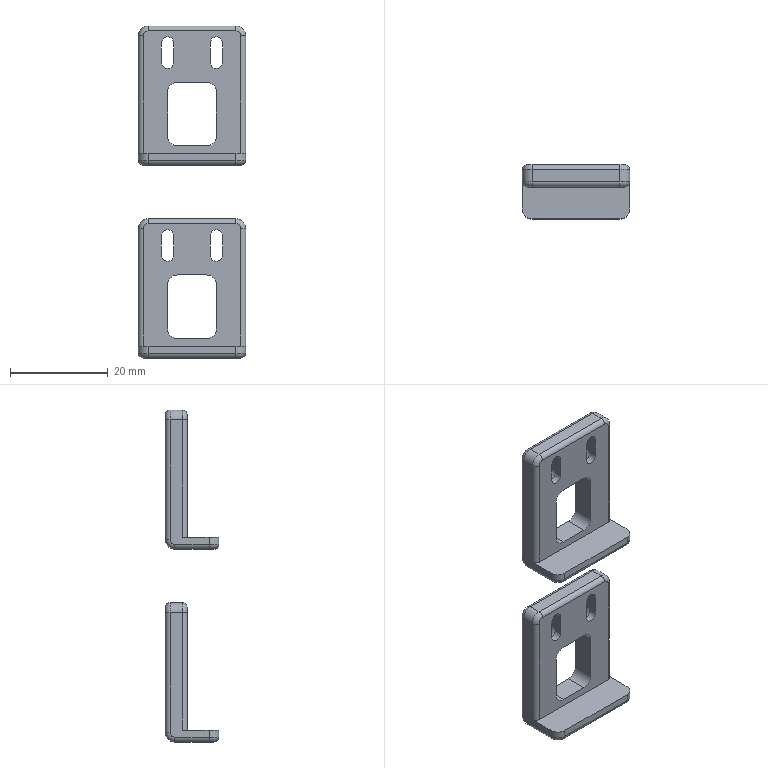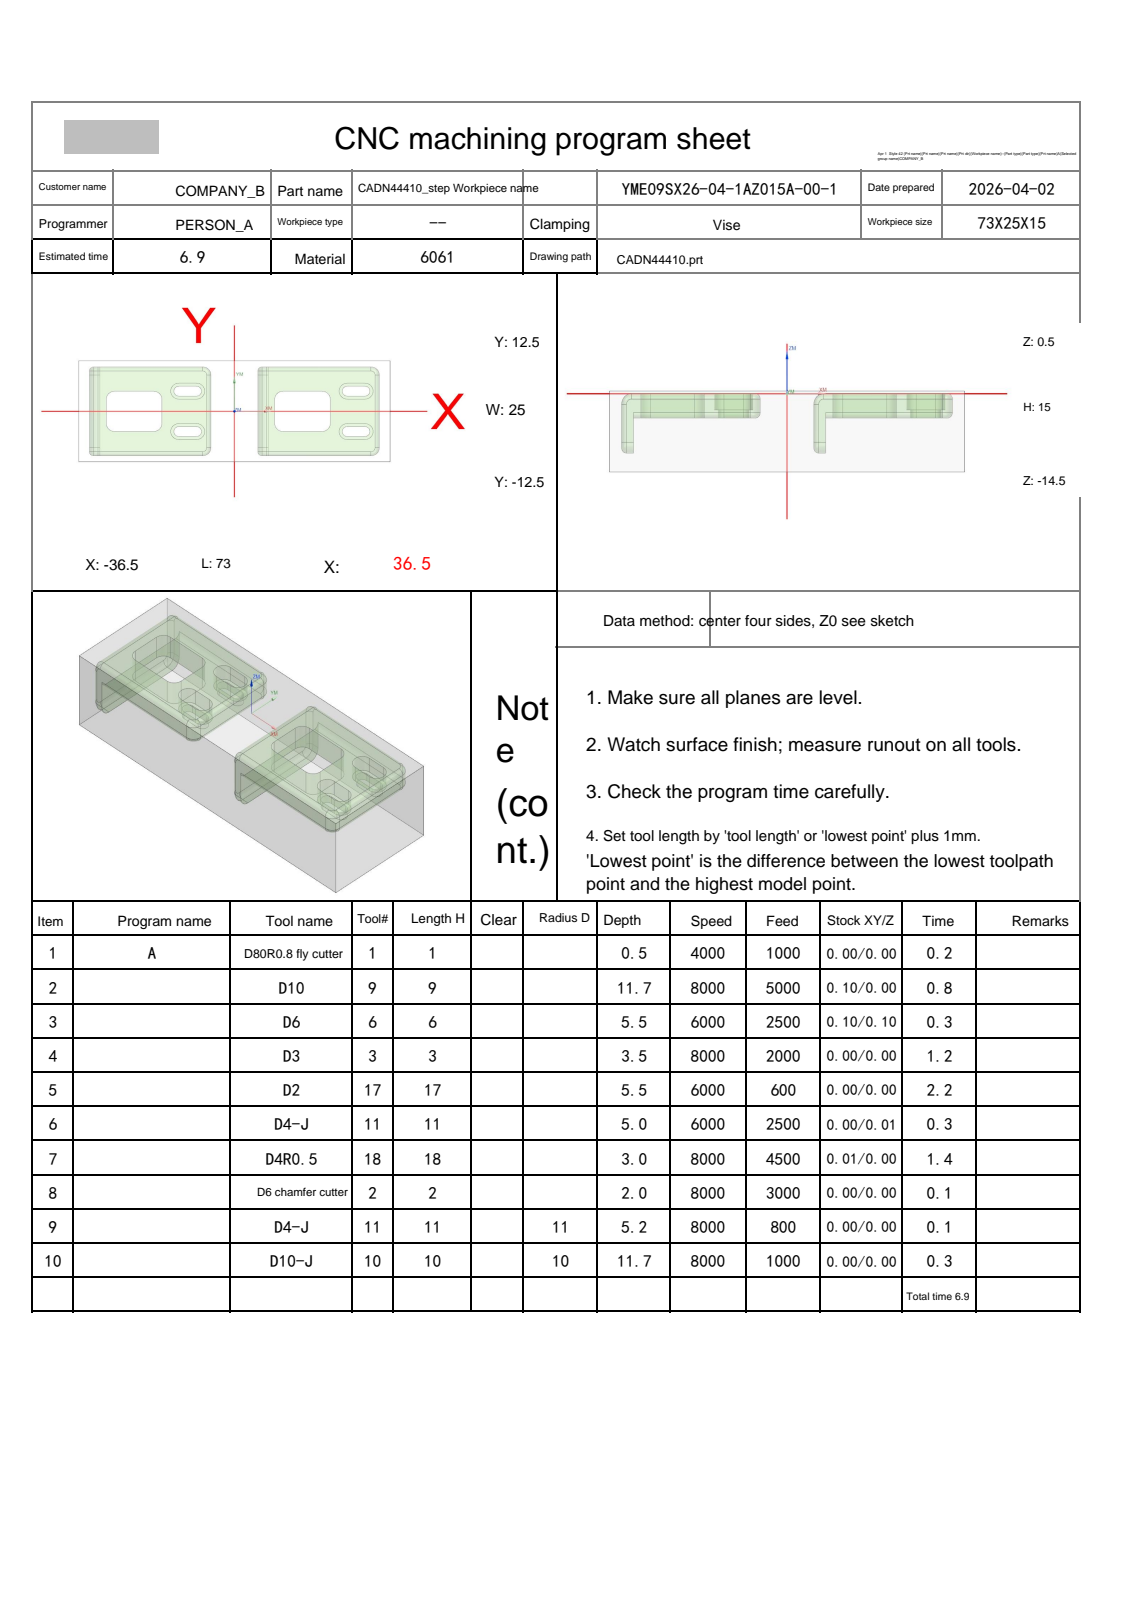NC program | NX | posted by the shop | part box 22 x 11 x 68 mm
Lines 970 to 2100 of 7842:
N4 T03 M06
(D3  D=3. R=0. H=03 ce=0.10 di=0.08)
G00 G90 G54 X-9.639 Y-4.6 M03 S8000
G43 H03 Z20.
M08
Z.8
G01 X-12.955 Z.626 F2000.
X-13.113 Z.618
X-13.355 Y-4.842 Z.6
Y-5.158 Z.583
X-13.113 Y-5.4 Z.565
X-8.798 Z.339
X-8.555 Y-5.158 Z.321
Y-4.842 Z.305
X-8.798 Y-4.6 Z.287
X-13.113 Z.061
X-13.355 Y-4.842 Z.043
Y-5.158 Z.026
X-13.113 Y-5.4 Z.008
X-12.955 Z0.0
X-8.955 Z-.037
G03 X-8.555 Y-5. Z-.043 I0.0 J.4
X-8.955 Y-4.6 Z-.049 I-.4 J0.0
G01 X-12.955 Z-.086
G03 X-13.355 Y-5. Z-.092 I0.0 J-.4
X-12.955 Y-5.4 Z-.098 I.4 J0.0
G01 X-8.955 Z-.135
G03 X-8.555 Y-5. Z-.141 I0.0 J.4
X-8.955 Y-4.6 Z-.147 I-.4 J0.0
G01 X-12.955 Z-.184
G03 X-13.355 Y-5. Z-.19 I0.0 J-.4
X-12.955 Y-5.4 Z-.196 I.4 J0.0
G01 X-8.955 Z-.233
G03 X-8.555 Y-5. Z-.239 I0.0 J.4
X-8.955 Y-4.6 Z-.245 I-.4 J0.0
G01 X-12.955 Z-.282
G03 X-13.355 Y-5. Z-.288 I0.0 J-.4
X-12.955 Y-5.4 Z-.294 I.4 J0.0
G01 X-8.955 Z-.331
G03 X-8.555 Y-5. Z-.337 I0.0 J.4
X-8.955 Y-4.6 Z-.343 I-.4 J0.0
G01 X-12.955 Z-.38
G03 X-13.355 Y-5. Z-.386 I0.0 J-.4
X-12.955 Y-5.4 Z-.392 I.4 J0.0
G01 X-8.955 Z-.429
G03 X-8.555 Y-5. Z-.435 I0.0 J.4
X-8.955 Y-4.6 Z-.441 I-.4 J0.0
G01 X-12.955 Z-.478
G03 X-13.355 Y-5. Z-.484 I0.0 J-.4
X-12.955 Y-5.4 Z-.49 I.4 J0.0
G01 X-8.955 Z-.527
G03 X-8.555 Y-5. Z-.533 I0.0 J.4
X-8.955 Y-4.6 Z-.539 I-.4 J0.0
G01 X-12.955 Z-.576
G03 X-13.355 Y-5. Z-.582 I0.0 J-.4
X-12.955 Y-5.4 Z-.588 I.4 J0.0
G01 X-8.955 Z-.625
G03 X-8.555 Y-5. Z-.631 I0.0 J.4
X-8.955 Y-4.6 Z-.637 I-.4 J0.0
G01 X-12.955 Z-.674
G03 X-13.355 Y-5. Z-.68 I0.0 J-.4
X-12.955 Y-5.4 Z-.686 I.4 J0.0
G01 X-8.955 Z-.723
G03 X-8.555 Y-5. Z-.729 I0.0 J.4
X-8.955 Y-4.6 Z-.735 I-.4 J0.0
G01 X-12.955 Z-.772
G03 X-13.355 Y-5. Z-.778 I0.0 J-.4
X-12.955 Y-5.4 Z-.784 I.4 J0.0
G01 X-8.955 Z-.821
G03 X-8.555 Y-5. Z-.827 I0.0 J.4
X-8.955 Y-4.6 Z-.833 I-.4 J0.0
G01 X-12.955 Z-.87
G03 X-13.355 Y-5. Z-.876 I0.0 J-.4
X-12.955 Y-5.4 Z-.882 I.4 J0.0
G01 X-8.955 Z-.919
G03 X-8.555 Y-5. Z-.925 I0.0 J.4
X-8.955 Y-4.6 Z-.931 I-.4 J0.0
G01 X-12.955 Z-.968
G03 X-13.355 Y-5. Z-.974 I0.0 J-.4
X-12.955 Y-5.4 Z-.98 I.4 J0.0
G01 X-8.955 Z-1.017
G03 X-8.555 Y-5. Z-1.023 I0.0 J.4
X-8.955 Y-4.6 Z-1.029 I-.4 J0.0
G01 X-12.955 Z-1.066
G03 X-13.355 Y-5. Z-1.072 I0.0 J-.4
X-12.955 Y-5.4 Z-1.078 I.4 J0.0
G01 X-8.955 Z-1.115
G03 X-8.555 Y-5. Z-1.121 I0.0 J.4
X-8.955 Y-4.6 Z-1.127 I-.4 J0.0
G01 X-12.955 Z-1.164
G03 X-13.355 Y-5. Z-1.17 I0.0 J-.4
X-12.955 Y-5.4 Z-1.176 I.4 J0.0
G01 X-8.955 Z-1.213
G03 X-8.555 Y-5. Z-1.219 I0.0 J.4
X-8.955 Y-4.6 Z-1.225 I-.4 J0.0
G01 X-12.955 Z-1.262
G03 X-13.355 Y-5. Z-1.268 I0.0 J-.4
X-12.955 Y-5.4 Z-1.274 I.4 J0.0
G01 X-8.955 Z-1.311
G03 X-8.555 Y-5. Z-1.317 I0.0 J.4
X-8.955 Y-4.6 Z-1.323 I-.4 J0.0
G01 X-12.955 Z-1.36
G03 X-13.355 Y-5. Z-1.366 I0.0 J-.4
X-12.955 Y-5.4 Z-1.372 I.4 J0.0
G01 X-8.955 Z-1.409
G03 X-8.555 Y-5. Z-1.415 I0.0 J.4
X-8.955 Y-4.6 Z-1.421 I-.4 J0.0
G01 X-12.955 Z-1.458
G03 X-13.355 Y-5. Z-1.464 I0.0 J-.4
X-12.955 Y-5.4 Z-1.47 I.4 J0.0
G01 X-8.955 Z-1.507
G03 X-8.555 Y-5. Z-1.513 I0.0 J.4
X-8.955 Y-4.6 Z-1.519 I-.4 J0.0
G01 X-12.955 Z-1.556
G03 X-13.355 Y-5. Z-1.562 I0.0 J-.4
X-12.955 Y-5.4 Z-1.568 I.4 J0.0
G01 X-8.955 Z-1.605
G03 X-8.555 Y-5. Z-1.611 I0.0 J.4
X-8.955 Y-4.6 Z-1.617 I-.4 J0.0
G01 X-12.955 Z-1.654
G03 X-13.355 Y-5. Z-1.66 I0.0 J-.4
X-12.955 Y-5.4 Z-1.666 I.4 J0.0
G01 X-8.955 Z-1.703
G03 X-8.555 Y-5. Z-1.709 I0.0 J.4
X-8.955 Y-4.6 Z-1.715 I-.4 J0.0
G01 X-12.955 Z-1.752
G03 X-13.355 Y-5. Z-1.758 I0.0 J-.4
X-12.955 Y-5.4 Z-1.764 I.4 J0.0
G01 X-8.955 Z-1.801
G03 X-8.555 Y-5. Z-1.807 I0.0 J.4
X-8.955 Y-4.6 Z-1.813 I-.4 J0.0
G01 X-12.955 Z-1.85
G03 X-13.355 Y-5. Z-1.856 I0.0 J-.4
X-12.955 Y-5.4 Z-1.862 I.4 J0.0
G01 X-8.955 Z-1.899
G03 X-8.555 Y-5. Z-1.905 I0.0 J.4
X-8.955 Y-4.6 Z-1.911 I-.4 J0.0
G01 X-12.955 Z-1.948
G03 X-13.355 Y-5. Z-1.954 I0.0 J-.4
X-12.955 Y-5.4 Z-1.96 I.4 J0.0
G01 X-8.955 Z-1.997
G03 X-8.555 Y-5. Z-2.003 I0.0 J.4
X-8.955 Y-4.6 Z-2.009 I-.4 J0.0
G01 X-12.955 Z-2.046
G03 X-13.355 Y-5. Z-2.052 I0.0 J-.4
X-12.955 Y-5.4 Z-2.058 I.4 J0.0
G01 X-8.955 Z-2.095
G03 X-8.555 Y-5. Z-2.101 I0.0 J.4
X-8.955 Y-4.6 Z-2.107 I-.4 J0.0
G01 X-12.955 Z-2.144
G03 X-13.355 Y-5. Z-2.15 I0.0 J-.4
X-12.955 Y-5.4 Z-2.156 I.4 J0.0
G01 X-8.955 Z-2.193
G03 X-8.555 Y-5. Z-2.199 I0.0 J.4
X-8.955 Y-4.6 Z-2.205 I-.4 J0.0
G01 X-12.955 Z-2.242
G03 X-13.355 Y-5. Z-2.248 I0.0 J-.4
X-12.955 Y-5.4 Z-2.254 I.4 J0.0
G01 X-8.955 Z-2.291
G03 X-8.555 Y-5. Z-2.297 I0.0 J.4
X-8.955 Y-4.6 Z-2.303 I-.4 J0.0
G01 X-12.955 Z-2.34
G03 X-13.355 Y-5. Z-2.346 I0.0 J-.4
X-12.955 Y-5.4 Z-2.352 I.4 J0.0
G01 X-8.955 Z-2.389
G03 X-8.555 Y-5. Z-2.395 I0.0 J.4
X-8.955 Y-4.6 Z-2.401 I-.4 J0.0
G01 X-12.955 Z-2.438
G03 X-13.355 Y-5. Z-2.444 I0.0 J-.4
X-12.955 Y-5.4 Z-2.45 I.4 J0.0
G01 X-8.955 Z-2.487
G03 X-8.555 Y-5. Z-2.493 I0.0 J.4
X-8.955 Y-4.6 Z-2.499 I-.4 J0.0
G01 X-12.955 Z-2.536
G03 X-13.355 Y-5. Z-2.542 I0.0 J-.4
X-12.955 Y-5.4 Z-2.548 I.4 J0.0
G01 X-8.955 Z-2.585
G03 X-8.555 Y-5. Z-2.591 I0.0 J.4
X-8.955 Y-4.6 Z-2.597 I-.4 J0.0
G01 X-12.955 Z-2.634
G03 X-13.355 Y-5. Z-2.64 I0.0 J-.4
X-12.955 Y-5.4 Z-2.646 I.4 J0.0
G01 X-8.955 Z-2.683
G03 X-8.555 Y-5. Z-2.689 I0.0 J.4
X-8.955 Y-4.6 Z-2.695 I-.4 J0.0
G01 X-12.955 Z-2.732
G03 X-13.355 Y-5. Z-2.738 I0.0 J-.4
X-12.955 Y-5.4 Z-2.744 I.4 J0.0
G01 X-8.955 Z-2.781
G03 X-8.555 Y-5. Z-2.787 I0.0 J.4
X-8.955 Y-4.6 Z-2.793 I-.4 J0.0
G01 X-12.955 Z-2.83
G03 X-13.355 Y-5. Z-2.836 I0.0 J-.4
X-12.955 Y-5.4 Z-2.842 I.4 J0.0
G01 X-8.955 Z-2.879
G03 X-8.555 Y-5. Z-2.885 I0.0 J.4
X-8.955 Y-4.6 Z-2.891 I-.4 J0.0
G01 X-12.955 Z-2.928
G03 X-13.355 Y-5. Z-2.934 I0.0 J-.4
X-12.955 Y-5.4 Z-2.94 I.4 J0.0
G01 X-8.955
G03 X-8.555 Y-5. I0.0 J.4
X-8.955 Y-4.6 I-.4 J0.0
G01 X-12.955
G03 X-13.355 Y-5. I0.0 J-.4
X-12.955 Y-5.4 I.4 J0.0
G01 X-12.555
Z-2.14
G00 Z20.
X-12.271 Y4.6
Z.8
G01 X-8.955 Z.626
X-8.798 Z.618
X-8.555 Y4.842 Z.6
Y5.158 Z.583
X-8.798 Y5.4 Z.565
X-13.113 Z.339
X-13.355 Y5.158 Z.321
Y4.842 Z.305
X-13.113 Y4.6 Z.287
X-8.798 Z.061
X-8.555 Y4.842 Z.043
Y5.158 Z.026
X-8.798 Y5.4 Z.008
X-8.955 Z0.0
X-12.955 Z-.037
G03 X-13.355 Y5. Z-.043 I0.0 J-.4
X-12.955 Y4.6 Z-.049 I.4 J0.0
G01 X-8.955 Z-.086
G03 X-8.555 Y5. Z-.092 I0.0 J.4
X-8.955 Y5.4 Z-.098 I-.4 J0.0
G01 X-12.955 Z-.135
G03 X-13.355 Y5. Z-.141 I0.0 J-.4
X-12.955 Y4.6 Z-.147 I.4 J0.0
G01 X-8.955 Z-.184
G03 X-8.555 Y5. Z-.19 I0.0 J.4
X-8.955 Y5.4 Z-.196 I-.4 J0.0
G01 X-12.955 Z-.233
G03 X-13.355 Y5. Z-.239 I0.0 J-.4
X-12.955 Y4.6 Z-.245 I.4 J0.0
G01 X-8.955 Z-.282
G03 X-8.555 Y5. Z-.288 I0.0 J.4
X-8.955 Y5.4 Z-.294 I-.4 J0.0
G01 X-12.955 Z-.331
G03 X-13.355 Y5. Z-.337 I0.0 J-.4
X-12.955 Y4.6 Z-.343 I.4 J0.0
G01 X-8.955 Z-.38
G03 X-8.555 Y5. Z-.386 I0.0 J.4
X-8.955 Y5.4 Z-.392 I-.4 J0.0
G01 X-12.955 Z-.429
G03 X-13.355 Y5. Z-.435 I0.0 J-.4
X-12.955 Y4.6 Z-.441 I.4 J0.0
G01 X-8.955 Z-.478
G03 X-8.555 Y5. Z-.484 I0.0 J.4
X-8.955 Y5.4 Z-.49 I-.4 J0.0
G01 X-12.955 Z-.527
G03 X-13.355 Y5. Z-.533 I0.0 J-.4
X-12.955 Y4.6 Z-.539 I.4 J0.0
G01 X-8.955 Z-.576
G03 X-8.555 Y5. Z-.582 I0.0 J.4
X-8.955 Y5.4 Z-.588 I-.4 J0.0
G01 X-12.955 Z-.625
G03 X-13.355 Y5. Z-.631 I0.0 J-.4
X-12.955 Y4.6 Z-.637 I.4 J0.0
G01 X-8.955 Z-.674
G03 X-8.555 Y5. Z-.68 I0.0 J.4
X-8.955 Y5.4 Z-.686 I-.4 J0.0
G01 X-12.955 Z-.723
G03 X-13.355 Y5. Z-.729 I0.0 J-.4
X-12.955 Y4.6 Z-.735 I.4 J0.0
G01 X-8.955 Z-.772
G03 X-8.555 Y5. Z-.778 I0.0 J.4
X-8.955 Y5.4 Z-.784 I-.4 J0.0
G01 X-12.955 Z-.821
G03 X-13.355 Y5. Z-.827 I0.0 J-.4
X-12.955 Y4.6 Z-.833 I.4 J0.0
G01 X-8.955 Z-.87
G03 X-8.555 Y5. Z-.876 I0.0 J.4
X-8.955 Y5.4 Z-.882 I-.4 J0.0
G01 X-12.955 Z-.919
G03 X-13.355 Y5. Z-.925 I0.0 J-.4
X-12.955 Y4.6 Z-.931 I.4 J0.0
G01 X-8.955 Z-.968
G03 X-8.555 Y5. Z-.974 I0.0 J.4
X-8.955 Y5.4 Z-.98 I-.4 J0.0
G01 X-12.955 Z-1.017
G03 X-13.355 Y5. Z-1.023 I0.0 J-.4
X-12.955 Y4.6 Z-1.029 I.4 J0.0
G01 X-8.955 Z-1.066
G03 X-8.555 Y5. Z-1.072 I0.0 J.4
X-8.955 Y5.4 Z-1.078 I-.4 J0.0
G01 X-12.955 Z-1.115
G03 X-13.355 Y5. Z-1.121 I0.0 J-.4
X-12.955 Y4.6 Z-1.127 I.4 J0.0
G01 X-8.955 Z-1.164
G03 X-8.555 Y5. Z-1.17 I0.0 J.4
X-8.955 Y5.4 Z-1.176 I-.4 J0.0
G01 X-12.955 Z-1.213
G03 X-13.355 Y5. Z-1.219 I0.0 J-.4
X-12.955 Y4.6 Z-1.225 I.4 J0.0
G01 X-8.955 Z-1.262
G03 X-8.555 Y5. Z-1.268 I0.0 J.4
X-8.955 Y5.4 Z-1.274 I-.4 J0.0
G01 X-12.955 Z-1.311
G03 X-13.355 Y5. Z-1.317 I0.0 J-.4
X-12.955 Y4.6 Z-1.323 I.4 J0.0
G01 X-8.955 Z-1.36
G03 X-8.555 Y5. Z-1.366 I0.0 J.4
X-8.955 Y5.4 Z-1.372 I-.4 J0.0
G01 X-12.955 Z-1.409
G03 X-13.355 Y5. Z-1.415 I0.0 J-.4
X-12.955 Y4.6 Z-1.421 I.4 J0.0
G01 X-8.955 Z-1.458
G03 X-8.555 Y5. Z-1.464 I0.0 J.4
X-8.955 Y5.4 Z-1.47 I-.4 J0.0
G01 X-12.955 Z-1.507
G03 X-13.355 Y5. Z-1.513 I0.0 J-.4
X-12.955 Y4.6 Z-1.519 I.4 J0.0
G01 X-8.955 Z-1.556
G03 X-8.555 Y5. Z-1.562 I0.0 J.4
X-8.955 Y5.4 Z-1.568 I-.4 J0.0
G01 X-12.955 Z-1.605
G03 X-13.355 Y5. Z-1.611 I0.0 J-.4
X-12.955 Y4.6 Z-1.617 I.4 J0.0
G01 X-8.955 Z-1.654
G03 X-8.555 Y5. Z-1.66 I0.0 J.4
X-8.955 Y5.4 Z-1.666 I-.4 J0.0
G01 X-12.955 Z-1.703
G03 X-13.355 Y5. Z-1.709 I0.0 J-.4
X-12.955 Y4.6 Z-1.715 I.4 J0.0
G01 X-8.955 Z-1.752
G03 X-8.555 Y5. Z-1.758 I0.0 J.4
X-8.955 Y5.4 Z-1.764 I-.4 J0.0
G01 X-12.955 Z-1.801
G03 X-13.355 Y5. Z-1.807 I0.0 J-.4
X-12.955 Y4.6 Z-1.813 I.4 J0.0
G01 X-8.955 Z-1.85
G03 X-8.555 Y5. Z-1.856 I0.0 J.4
X-8.955 Y5.4 Z-1.862 I-.4 J0.0
G01 X-12.955 Z-1.899
G03 X-13.355 Y5. Z-1.905 I0.0 J-.4
X-12.955 Y4.6 Z-1.911 I.4 J0.0
G01 X-8.955 Z-1.948
G03 X-8.555 Y5. Z-1.954 I0.0 J.4
X-8.955 Y5.4 Z-1.96 I-.4 J0.0
G01 X-12.955 Z-1.997
G03 X-13.355 Y5. Z-2.003 I0.0 J-.4
X-12.955 Y4.6 Z-2.009 I.4 J0.0
G01 X-8.955 Z-2.046
G03 X-8.555 Y5. Z-2.052 I0.0 J.4
X-8.955 Y5.4 Z-2.058 I-.4 J0.0
G01 X-12.955 Z-2.095
G03 X-13.355 Y5. Z-2.101 I0.0 J-.4
X-12.955 Y4.6 Z-2.107 I.4 J0.0
G01 X-8.955 Z-2.144
G03 X-8.555 Y5. Z-2.15 I0.0 J.4
X-8.955 Y5.4 Z-2.156 I-.4 J0.0
G01 X-12.955 Z-2.193
G03 X-13.355 Y5. Z-2.199 I0.0 J-.4
X-12.955 Y4.6 Z-2.205 I.4 J0.0
G01 X-8.955 Z-2.242
G03 X-8.555 Y5. Z-2.248 I0.0 J.4
X-8.955 Y5.4 Z-2.254 I-.4 J0.0
G01 X-12.955 Z-2.291
G03 X-13.355 Y5. Z-2.297 I0.0 J-.4
X-12.955 Y4.6 Z-2.303 I.4 J0.0
G01 X-8.955 Z-2.34
G03 X-8.555 Y5. Z-2.346 I0.0 J.4
X-8.955 Y5.4 Z-2.352 I-.4 J0.0
G01 X-12.955 Z-2.389
G03 X-13.355 Y5. Z-2.395 I0.0 J-.4
X-12.955 Y4.6 Z-2.401 I.4 J0.0
G01 X-8.955 Z-2.438
G03 X-8.555 Y5. Z-2.444 I0.0 J.4
X-8.955 Y5.4 Z-2.45 I-.4 J0.0
G01 X-12.955 Z-2.487
G03 X-13.355 Y5. Z-2.493 I0.0 J-.4
X-12.955 Y4.6 Z-2.499 I.4 J0.0
G01 X-8.955 Z-2.536
G03 X-8.555 Y5. Z-2.542 I0.0 J.4
X-8.955 Y5.4 Z-2.548 I-.4 J0.0
G01 X-12.955 Z-2.585
G03 X-13.355 Y5. Z-2.591 I0.0 J-.4
X-12.955 Y4.6 Z-2.597 I.4 J0.0
G01 X-8.955 Z-2.634
G03 X-8.555 Y5. Z-2.64 I0.0 J.4
X-8.955 Y5.4 Z-2.646 I-.4 J0.0
G01 X-12.955 Z-2.683
G03 X-13.355 Y5. Z-2.689 I0.0 J-.4
X-12.955 Y4.6 Z-2.695 I.4 J0.0
G01 X-8.955 Z-2.732
G03 X-8.555 Y5. Z-2.738 I0.0 J.4
X-8.955 Y5.4 Z-2.744 I-.4 J0.0
G01 X-12.955 Z-2.781
G03 X-13.355 Y5. Z-2.787 I0.0 J-.4
X-12.955 Y4.6 Z-2.793 I.4 J0.0
G01 X-8.955 Z-2.83
G03 X-8.555 Y5. Z-2.836 I0.0 J.4
X-8.955 Y5.4 Z-2.842 I-.4 J0.0
G01 X-12.955 Z-2.879
G03 X-13.355 Y5. Z-2.885 I0.0 J-.4
X-12.955 Y4.6 Z-2.891 I.4 J0.0
G01 X-8.955 Z-2.928
G03 X-8.555 Y5. Z-2.934 I0.0 J.4
X-8.955 Y5.4 Z-2.94 I-.4 J0.0
G01 X-12.955
G03 X-13.355 Y5. I0.0 J-.4
X-12.955 Y4.6 I.4 J0.0
G01 X-8.955
G03 X-8.555 Y5. I0.0 J.4
X-8.955 Y5.4 I-.4 J0.0
G01 X-9.355
Z-2.14
G00 Z20.
X27.229 Y-5.4
Z.8
G01 X30.545 Z.626
X30.702 Z.618
X30.945 Y-5.158 Z.6
Y-4.842 Z.583
X30.702 Y-4.6 Z.565
X26.387 Z.339
X26.145 Y-4.842 Z.321
Y-5.158 Z.305
X26.387 Y-5.4 Z.287
X30.702 Z.061
X30.945 Y-5.158 Z.043
Y-4.842 Z.026
X30.702 Y-4.6 Z.008
X30.545 Z0.0
X26.545 Z-.037
G03 X26.145 Y-5. Z-.043 I0.0 J-.4
X26.545 Y-5.4 Z-.049 I.4 J0.0
G01 X30.545 Z-.086
G03 X30.945 Y-5. Z-.092 I0.0 J.4
X30.545 Y-4.6 Z-.098 I-.4 J0.0
G01 X26.545 Z-.135
G03 X26.145 Y-5. Z-.141 I0.0 J-.4
X26.545 Y-5.4 Z-.147 I.4 J0.0
G01 X30.545 Z-.184
G03 X30.945 Y-5. Z-.19 I0.0 J.4
X30.545 Y-4.6 Z-.196 I-.4 J0.0
G01 X26.545 Z-.233
G03 X26.145 Y-5. Z-.239 I0.0 J-.4
X26.545 Y-5.4 Z-.245 I.4 J0.0
G01 X30.545 Z-.282
G03 X30.945 Y-5. Z-.288 I0.0 J.4
X30.545 Y-4.6 Z-.294 I-.4 J0.0
G01 X26.545 Z-.331
G03 X26.145 Y-5. Z-.337 I0.0 J-.4
X26.545 Y-5.4 Z-.343 I.4 J0.0
G01 X30.545 Z-.38
G03 X30.945 Y-5. Z-.386 I0.0 J.4
X30.545 Y-4.6 Z-.392 I-.4 J0.0
G01 X26.545 Z-.429
G03 X26.145 Y-5. Z-.435 I0.0 J-.4
X26.545 Y-5.4 Z-.441 I.4 J0.0
G01 X30.545 Z-.478
G03 X30.945 Y-5. Z-.484 I0.0 J.4
X30.545 Y-4.6 Z-.49 I-.4 J0.0
G01 X26.545 Z-.527
G03 X26.145 Y-5. Z-.533 I0.0 J-.4
X26.545 Y-5.4 Z-.539 I.4 J0.0
G01 X30.545 Z-.576
G03 X30.945 Y-5. Z-.582 I0.0 J.4
X30.545 Y-4.6 Z-.588 I-.4 J0.0
G01 X26.545 Z-.625
G03 X26.145 Y-5. Z-.631 I0.0 J-.4
X26.545 Y-5.4 Z-.637 I.4 J0.0
G01 X30.545 Z-.674
G03 X30.945 Y-5. Z-.68 I0.0 J.4
X30.545 Y-4.6 Z-.686 I-.4 J0.0
G01 X26.545 Z-.723
G03 X26.145 Y-5. Z-.729 I0.0 J-.4
X26.545 Y-5.4 Z-.735 I.4 J0.0
G01 X30.545 Z-.772
G03 X30.945 Y-5. Z-.778 I0.0 J.4
X30.545 Y-4.6 Z-.784 I-.4 J0.0
G01 X26.545 Z-.821
G03 X26.145 Y-5. Z-.827 I0.0 J-.4
X26.545 Y-5.4 Z-.833 I.4 J0.0
G01 X30.545 Z-.87
G03 X30.945 Y-5. Z-.876 I0.0 J.4
X30.545 Y-4.6 Z-.882 I-.4 J0.0
G01 X26.545 Z-.919
G03 X26.145 Y-5. Z-.925 I0.0 J-.4
X26.545 Y-5.4 Z-.931 I.4 J0.0
G01 X30.545 Z-.968
G03 X30.945 Y-5. Z-.974 I0.0 J.4
X30.545 Y-4.6 Z-.98 I-.4 J0.0
G01 X26.545 Z-1.017
G03 X26.145 Y-5. Z-1.023 I0.0 J-.4
X26.545 Y-5.4 Z-1.029 I.4 J0.0
G01 X30.545 Z-1.066
G03 X30.945 Y-5. Z-1.072 I0.0 J.4
X30.545 Y-4.6 Z-1.078 I-.4 J0.0
G01 X26.545 Z-1.115
G03 X26.145 Y-5. Z-1.121 I0.0 J-.4
X26.545 Y-5.4 Z-1.127 I.4 J0.0
G01 X30.545 Z-1.164
G03 X30.945 Y-5. Z-1.17 I0.0 J.4
X30.545 Y-4.6 Z-1.176 I-.4 J0.0
G01 X26.545 Z-1.213
G03 X26.145 Y-5. Z-1.219 I0.0 J-.4
X26.545 Y-5.4 Z-1.225 I.4 J0.0
G01 X30.545 Z-1.262
G03 X30.945 Y-5. Z-1.268 I0.0 J.4
X30.545 Y-4.6 Z-1.274 I-.4 J0.0
G01 X26.545 Z-1.311
G03 X26.145 Y-5. Z-1.317 I0.0 J-.4
X26.545 Y-5.4 Z-1.323 I.4 J0.0
G01 X30.545 Z-1.36
G03 X30.945 Y-5. Z-1.366 I0.0 J.4
X30.545 Y-4.6 Z-1.372 I-.4 J0.0
G01 X26.545 Z-1.409
G03 X26.145 Y-5. Z-1.415 I0.0 J-.4
X26.545 Y-5.4 Z-1.421 I.4 J0.0
G01 X30.545 Z-1.458
G03 X30.945 Y-5. Z-1.464 I0.0 J.4
X30.545 Y-4.6 Z-1.47 I-.4 J0.0
G01 X26.545 Z-1.507
G03 X26.145 Y-5. Z-1.513 I0.0 J-.4
X26.545 Y-5.4 Z-1.519 I.4 J0.0
G01 X30.545 Z-1.556
G03 X30.945 Y-5. Z-1.562 I0.0 J.4
X30.545 Y-4.6 Z-1.568 I-.4 J0.0
G01 X26.545 Z-1.605
G03 X26.145 Y-5. Z-1.611 I0.0 J-.4
X26.545 Y-5.4 Z-1.617 I.4 J0.0
G01 X30.545 Z-1.654
G03 X30.945 Y-5. Z-1.66 I0.0 J.4
X30.545 Y-4.6 Z-1.666 I-.4 J0.0
G01 X26.545 Z-1.703
G03 X26.145 Y-5. Z-1.709 I0.0 J-.4
X26.545 Y-5.4 Z-1.715 I.4 J0.0
G01 X30.545 Z-1.752
G03 X30.945 Y-5. Z-1.758 I0.0 J.4
X30.545 Y-4.6 Z-1.764 I-.4 J0.0
G01 X26.545 Z-1.801
G03 X26.145 Y-5. Z-1.807 I0.0 J-.4
X26.545 Y-5.4 Z-1.813 I.4 J0.0
G01 X30.545 Z-1.85
G03 X30.945 Y-5. Z-1.856 I0.0 J.4
X30.545 Y-4.6 Z-1.862 I-.4 J0.0
G01 X26.545 Z-1.899
G03 X26.145 Y-5. Z-1.905 I0.0 J-.4
X26.545 Y-5.4 Z-1.911 I.4 J0.0
G01 X30.545 Z-1.948
G03 X30.945 Y-5. Z-1.954 I0.0 J.4
X30.545 Y-4.6 Z-1.96 I-.4 J0.0
G01 X26.545 Z-1.997
G03 X26.145 Y-5. Z-2.003 I0.0 J-.4
X26.545 Y-5.4 Z-2.009 I.4 J0.0
G01 X30.545 Z-2.046
G03 X30.945 Y-5. Z-2.052 I0.0 J.4
X30.545 Y-4.6 Z-2.058 I-.4 J0.0
G01 X26.545 Z-2.095
G03 X26.145 Y-5. Z-2.101 I0.0 J-.4
X26.545 Y-5.4 Z-2.107 I.4 J0.0
G01 X30.545 Z-2.144
G03 X30.945 Y-5. Z-2.15 I0.0 J.4
X30.545 Y-4.6 Z-2.156 I-.4 J0.0
G01 X26.545 Z-2.193
G03 X26.145 Y-5. Z-2.199 I0.0 J-.4
X26.545 Y-5.4 Z-2.205 I.4 J0.0
G01 X30.545 Z-2.242
G03 X30.945 Y-5. Z-2.248 I0.0 J.4
X30.545 Y-4.6 Z-2.254 I-.4 J0.0
G01 X26.545 Z-2.291
G03 X26.145 Y-5. Z-2.297 I0.0 J-.4
X26.545 Y-5.4 Z-2.303 I.4 J0.0
G01 X30.545 Z-2.34
G03 X30.945 Y-5. Z-2.346 I0.0 J.4
X30.545 Y-4.6 Z-2.352 I-.4 J0.0
G01 X26.545 Z-2.389
G03 X26.145 Y-5. Z-2.395 I0.0 J-.4
X26.545 Y-5.4 Z-2.401 I.4 J0.0
G01 X30.545 Z-2.438
G03 X30.945 Y-5. Z-2.444 I0.0 J.4
X30.545 Y-4.6 Z-2.45 I-.4 J0.0
G01 X26.545 Z-2.487
G03 X26.145 Y-5. Z-2.493 I0.0 J-.4
X26.545 Y-5.4 Z-2.499 I.4 J0.0
G01 X30.545 Z-2.536
G03 X30.945 Y-5. Z-2.542 I0.0 J.4
X30.545 Y-4.6 Z-2.548 I-.4 J0.0
G01 X26.545 Z-2.585
G03 X26.145 Y-5. Z-2.591 I0.0 J-.4
X26.545 Y-5.4 Z-2.597 I.4 J0.0
G01 X30.545 Z-2.634
G03 X30.945 Y-5. Z-2.64 I0.0 J.4
X30.545 Y-4.6 Z-2.646 I-.4 J0.0
G01 X26.545 Z-2.683
G03 X26.145 Y-5. Z-2.689 I0.0 J-.4
X26.545 Y-5.4 Z-2.695 I.4 J0.0
G01 X30.545 Z-2.732
G03 X30.945 Y-5. Z-2.738 I0.0 J.4
X30.545 Y-4.6 Z-2.744 I-.4 J0.0
G01 X26.545 Z-2.781
G03 X26.145 Y-5. Z-2.787 I0.0 J-.4
X26.545 Y-5.4 Z-2.793 I.4 J0.0
G01 X30.545 Z-2.83
G03 X30.945 Y-5. Z-2.836 I0.0 J.4
X30.545 Y-4.6 Z-2.842 I-.4 J0.0
G01 X26.545 Z-2.879
G03 X26.145 Y-5. Z-2.885 I0.0 J-.4
X26.545 Y-5.4 Z-2.891 I.4 J0.0
G01 X30.545 Z-2.928
G03 X30.945 Y-5. Z-2.934 I0.0 J.4
X30.545 Y-4.6 Z-2.94 I-.4 J0.0
G01 X26.545
G03 X26.145 Y-5. I0.0 J-.4
X26.545 Y-5.4 I.4 J0.0
G01 X30.545
G03 X30.945 Y-5. I0.0 J.4
X30.545 Y-4.6 I-.4 J0.0
G01 X30.145
Z-2.14
G00 Z20.
X29.861 Y5.4
Z.8
G01 X26.545 Z.626
X26.387 Z.618
X26.145 Y5.158 Z.6
Y4.842 Z.583
X26.387 Y4.6 Z.565
X30.702 Z.339
X30.945 Y4.842 Z.321
Y5.158 Z.305
X30.702 Y5.4 Z.287
X26.387 Z.061
X26.145 Y5.158 Z.043
Y4.842 Z.026
X26.387 Y4.6 Z.008
X26.545 Z0.0
X30.545 Z-.037
G03 X30.945 Y5. Z-.043 I0.0 J.4
X30.545 Y5.4 Z-.049 I-.4 J0.0
G01 X26.545 Z-.086
G03 X26.145 Y5. Z-.092 I0.0 J-.4
X26.545 Y4.6 Z-.098 I.4 J0.0
G01 X30.545 Z-.135
G03 X30.945 Y5. Z-.141 I0.0 J.4
X30.545 Y5.4 Z-.147 I-.4 J0.0
G01 X26.545 Z-.184
G03 X26.145 Y5. Z-.19 I0.0 J-.4
X26.545 Y4.6 Z-.196 I.4 J0.0
G01 X30.545 Z-.233
G03 X30.945 Y5. Z-.239 I0.0 J.4
X30.545 Y5.4 Z-.245 I-.4 J0.0
G01 X26.545 Z-.282
G03 X26.145 Y5. Z-.288 I0.0 J-.4
X26.545 Y4.6 Z-.294 I.4 J0.0
G01 X30.545 Z-.331
G03 X30.945 Y5. Z-.337 I0.0 J.4
X30.545 Y5.4 Z-.343 I-.4 J0.0
G01 X26.545 Z-.38
G03 X26.145 Y5. Z-.386 I0.0 J-.4
X26.545 Y4.6 Z-.392 I.4 J0.0
G01 X30.545 Z-.429
G03 X30.945 Y5. Z-.435 I0.0 J.4
X30.545 Y5.4 Z-.441 I-.4 J0.0
G01 X26.545 Z-.478
G03 X26.145 Y5. Z-.484 I0.0 J-.4
X26.545 Y4.6 Z-.49 I.4 J0.0
G01 X30.545 Z-.527
G03 X30.945 Y5. Z-.533 I0.0 J.4
X30.545 Y5.4 Z-.539 I-.4 J0.0
G01 X26.545 Z-.576
G03 X26.145 Y5. Z-.582 I0.0 J-.4
X26.545 Y4.6 Z-.588 I.4 J0.0
G01 X30.545 Z-.625
G03 X30.945 Y5. Z-.631 I0.0 J.4
X30.545 Y5.4 Z-.637 I-.4 J0.0
G01 X26.545 Z-.674
G03 X26.145 Y5. Z-.68 I0.0 J-.4
X26.545 Y4.6 Z-.686 I.4 J0.0
G01 X30.545 Z-.723
G03 X30.945 Y5. Z-.729 I0.0 J.4
X30.545 Y5.4 Z-.735 I-.4 J0.0
G01 X26.545 Z-.772
G03 X26.145 Y5. Z-.778 I0.0 J-.4
X26.545 Y4.6 Z-.784 I.4 J0.0
G01 X30.545 Z-.821
G03 X30.945 Y5. Z-.827 I0.0 J.4
X30.545 Y5.4 Z-.833 I-.4 J0.0
G01 X26.545 Z-.87
G03 X26.145 Y5. Z-.876 I0.0 J-.4
X26.545 Y4.6 Z-.882 I.4 J0.0
G01 X30.545 Z-.919
G03 X30.945 Y5. Z-.925 I0.0 J.4
X30.545 Y5.4 Z-.931 I-.4 J0.0
G01 X26.545 Z-.968
G03 X26.145 Y5. Z-.974 I0.0 J-.4
X26.545 Y4.6 Z-.98 I.4 J0.0
G01 X30.545 Z-1.017
G03 X30.945 Y5. Z-1.023 I0.0 J.4
X30.545 Y5.4 Z-1.029 I-.4 J0.0
G01 X26.545 Z-1.066
G03 X26.145 Y5. Z-1.072 I0.0 J-.4
X26.545 Y4.6 Z-1.078 I.4 J0.0
G01 X30.545 Z-1.115
G03 X30.945 Y5. Z-1.121 I0.0 J.4
X30.545 Y5.4 Z-1.127 I-.4 J0.0
G01 X26.545 Z-1.164
G03 X26.145 Y5. Z-1.17 I0.0 J-.4
X26.545 Y4.6 Z-1.176 I.4 J0.0
G01 X30.545 Z-1.213
G03 X30.945 Y5. Z-1.219 I0.0 J.4
X30.545 Y5.4 Z-1.225 I-.4 J0.0
G01 X26.545 Z-1.262
G03 X26.145 Y5. Z-1.268 I0.0 J-.4
X26.545 Y4.6 Z-1.274 I.4 J0.0
G01 X30.545 Z-1.311
G03 X30.945 Y5. Z-1.317 I0.0 J.4
X30.545 Y5.4 Z-1.323 I-.4 J0.0
G01 X26.545 Z-1.36
G03 X26.145 Y5. Z-1.366 I0.0 J-.4
X26.545 Y4.6 Z-1.372 I.4 J0.0
G01 X30.545 Z-1.409
G03 X30.945 Y5. Z-1.415 I0.0 J.4
X30.545 Y5.4 Z-1.421 I-.4 J0.0
G01 X26.545 Z-1.458
G03 X26.145 Y5. Z-1.464 I0.0 J-.4
X26.545 Y4.6 Z-1.47 I.4 J0.0
G01 X30.545 Z-1.507
G03 X30.945 Y5. Z-1.513 I0.0 J.4
X30.545 Y5.4 Z-1.519 I-.4 J0.0
G01 X26.545 Z-1.556
G03 X26.145 Y5. Z-1.562 I0.0 J-.4
X26.545 Y4.6 Z-1.568 I.4 J0.0
G01 X30.545 Z-1.605
G03 X30.945 Y5. Z-1.611 I0.0 J.4
X30.545 Y5.4 Z-1.617 I-.4 J0.0
G01 X26.545 Z-1.654
G03 X26.145 Y5. Z-1.66 I0.0 J-.4
X26.545 Y4.6 Z-1.666 I.4 J0.0
G01 X30.545 Z-1.703
G03 X30.945 Y5. Z-1.709 I0.0 J.4
X30.545 Y5.4 Z-1.715 I-.4 J0.0
G01 X26.545 Z-1.752
G03 X26.145 Y5. Z-1.758 I0.0 J-.4
X26.545 Y4.6 Z-1.764 I.4 J0.0
G01 X30.545 Z-1.801
G03 X30.945 Y5. Z-1.807 I0.0 J.4
X30.545 Y5.4 Z-1.813 I-.4 J0.0
G01 X26.545 Z-1.85
G03 X26.145 Y5. Z-1.856 I0.0 J-.4
X26.545 Y4.6 Z-1.862 I.4 J0.0
G01 X30.545 Z-1.899
G03 X30.945 Y5. Z-1.905 I0.0 J.4
X30.545 Y5.4 Z-1.911 I-.4 J0.0
G01 X26.545 Z-1.948
G03 X26.145 Y5. Z-1.954 I0.0 J-.4
X26.545 Y4.6 Z-1.96 I.4 J0.0
G01 X30.545 Z-1.997
G03 X30.945 Y5. Z-2.003 I0.0 J.4
X30.545 Y5.4 Z-2.009 I-.4 J0.0
G01 X26.545 Z-2.046
G03 X26.145 Y5. Z-2.052 I0.0 J-.4
X26.545 Y4.6 Z-2.058 I.4 J0.0
G01 X30.545 Z-2.095
G03 X30.945 Y5. Z-2.101 I0.0 J.4
X30.545 Y5.4 Z-2.107 I-.4 J0.0
G01 X26.545 Z-2.144
G03 X26.145 Y5. Z-2.15 I0.0 J-.4
X26.545 Y4.6 Z-2.156 I.4 J0.0
G01 X30.545 Z-2.193
G03 X30.945 Y5. Z-2.199 I0.0 J.4
X30.545 Y5.4 Z-2.205 I-.4 J0.0
G01 X26.545 Z-2.242
G03 X26.145 Y5. Z-2.248 I0.0 J-.4
X26.545 Y4.6 Z-2.254 I.4 J0.0
G01 X30.545 Z-2.291
G03 X30.945 Y5. Z-2.297 I0.0 J.4
X30.545 Y5.4 Z-2.303 I-.4 J0.0
G01 X26.545 Z-2.34
G03 X26.145 Y5. Z-2.346 I0.0 J-.4
X26.545 Y4.6 Z-2.352 I.4 J0.0
G01 X30.545 Z-2.389
G03 X30.945 Y5. Z-2.395 I0.0 J.4
X30.545 Y5.4 Z-2.401 I-.4 J0.0
G01 X26.545 Z-2.438
G03 X26.145 Y5. Z-2.444 I0.0 J-.4
X26.545 Y4.6 Z-2.45 I.4 J0.0
G01 X30.545 Z-2.487
G03 X30.945 Y5. Z-2.493 I0.0 J.4
X30.545 Y5.4 Z-2.499 I-.4 J0.0
G01 X26.545 Z-2.536
G03 X26.145 Y5. Z-2.542 I0.0 J-.4
X26.545 Y4.6 Z-2.548 I.4 J0.0
G01 X30.545 Z-2.585
G03 X30.945 Y5. Z-2.591 I0.0 J.4
X30.545 Y5.4 Z-2.597 I-.4 J0.0
G01 X26.545 Z-2.634
G03 X26.145 Y5. Z-2.64 I0.0 J-.4
X26.545 Y4.6 Z-2.646 I.4 J0.0
G01 X30.545 Z-2.683
G03 X30.945 Y5. Z-2.689 I0.0 J.4
X30.545 Y5.4 Z-2.695 I-.4 J0.0
G01 X26.545 Z-2.732
G03 X26.145 Y5. Z-2.738 I0.0 J-.4
X26.545 Y4.6 Z-2.744 I.4 J0.0
G01 X30.545 Z-2.781
G03 X30.945 Y5. Z-2.787 I0.0 J.4
X30.545 Y5.4 Z-2.793 I-.4 J0.0
G01 X26.545 Z-2.83
G03 X26.145 Y5. Z-2.836 I0.0 J-.4
X26.545 Y4.6 Z-2.842 I.4 J0.0
G01 X30.545 Z-2.879
G03 X30.945 Y5. Z-2.885 I0.0 J.4
X30.545 Y5.4 Z-2.891 I-.4 J0.0
G01 X26.545 Z-2.928
G03 X26.145 Y5. Z-2.934 I0.0 J-.4
X26.545 Y4.6 Z-2.94 I.4 J0.0
G01 X30.545
G03 X30.945 Y5. I0.0 J.4
X30.545 Y5.4 I-.4 J0.0
G01 X26.545
G03 X26.145 Y5. I0.0 J-.4
X26.545 Y4.6 I.4 J0.0
G01 X26.945
Z-2.14
G00 Z20.
G00 G90 X-11.155 Y-5.25 M03 S6000
Z20.
Z-2.5
G01 Z-3. F500.
G41 D03
Y-5.3
G03 X-10.955 Y-5.5 I.2 J0.0
G01 X-8.955
G03 X-8.455 Y-5. I0.0 J.5
X-8.955 Y-4.5 I-.5 J0.0
G01 X-12.955
G03 X-13.455 Y-5. I0.0 J-.5
X-12.955 Y-5.5 I.5 J0.0
G01 X-10.955
X-10.455
G03 X-10.255 Y-5.3 I0.0 J.2
G01 G40 Y-5.25
Z-2.5
G00 Z20.
X-10.755 Y5.25
Z-2.5
G01 Z-3.
G41 D03
Y5.3
G03 X-10.955 Y5.5 I-.2 J0.0
G01 X-12.955
G03 X-13.455 Y5. I0.0 J-.5
X-12.955 Y4.5 I.5 J0.0
G01 X-8.955
G03 X-8.455 Y5. I0.0 J.5
X-8.955 Y5.5 I-.5 J0.0
G01 X-10.955
X-11.455
G03 X-11.655 Y5.3 I0.0 J-.2
G01 G40 Y5.25
Z-2.5
G00 Z20.
X28.745 Y-4.75
Z-2.5
G01 Z-3.
G41 D03
Y-4.7
G03 X28.545 Y-4.5 I-.2 J0.0
G01 X26.545
G03 X26.045 Y-5. I0.0 J-.5
X26.545 Y-5.5 I.5 J0.0
G01 X30.545
G03 X31.045 Y-5. I0.0 J.5
X30.545 Y-4.5 I-.5 J0.0
G01 X28.545
X28.045
G03 X27.845 Y-4.7 I0.0 J-.2
G01 G40 Y-4.75
Z-2.5
G00 Z20.
X28.745 Y5.25
Z-2.5
G01 Z-3.
G41 D03
Y5.3
G03 X28.545 Y5.5 I-.2 J0.0
G01 X26.545
G03 X26.045 Y5. I0.0 J-.5
X26.545 Y4.5 I.5 J0.0
G01 X30.545
G03 X31.045 Y5. I0.0 J.5
X30.545 Y5.5 I-.5 J0.0
G01 X28.545
X28.045
G03 X27.845 Y5.3 I0.0 J-.2
G01 G40 Y5.25
Z-2.5
G00 Z20.
G00 G90 X-11.586 Y-5.466 M03 S8000
Z20.
Z.5
G01 X-8.887 Z.359 F600.
X-8.744 Y-5.421 Z.351
X-8.622 Y-5.333 Z.343
X-8.534 Y-5.211 Z.335
X-8.489 Y-5.068 Z.327
Y-4.932 Z.32
X-8.534 Y-4.789 Z.312
X-8.622 Y-4.667 Z.304
X-8.744 Y-4.579 Z.296
X-8.887 Y-4.534 Z.289
X-13.024 Z.072
X-13.167 Y-4.579 Z.064
X-13.288 Y-4.667 Z.056
X-13.376 Y-4.789 Z.048
X-13.421 Y-4.932 Z.04
Y-5.068 Z.033
X-13.358 Y-5.245 Z.023
X-13.23 Y-5.383 Z.013
X-13.059 Y-5.459 Z.004
X-12.991 Y-5.465 Z0.0
G41 D03
X-12.955 Y-5.5
X-8.955 Z-.359
G03 X-8.455 Y-5. Z-.43 I0.0 J.5
X-8.955 Y-4.5 Z-.5 I-.5 J0.0
G01 X-12.955 Z-.859
G03 X-13.455 Y-5. Z-.93 I0.0 J-.5
X-12.955 Y-5.5 Z-1. I.5 J0.0
G01 X-8.955 Z-1.359
G03 X-8.455 Y-5. Z-1.43 I0.0 J.5
X-8.955 Y-4.5 Z-1.5 I-.5 J0.0
G01 X-12.955 Z-1.859
G03 X-13.455 Y-5. Z-1.93 I0.0 J-.5
X-12.955 Y-5.5 Z-2. I.5 J0.0
G01 X-8.955 Z-2.359
G03 X-8.455 Y-5. Z-2.43 I0.0 J.5
X-8.955 Y-4.5 Z-2.5 I-.5 J0.0
G01 X-12.955 Z-2.859
G03 X-13.455 Y-5. Z-2.93 I0.0 J-.5
X-12.955 Y-5.5 Z-3. I.5 J0.0
G01 X-8.955
G03 X-8.455 Y-5. I0.0 J.5
X-8.955 Y-4.5 I-.5 J0.0
G01 X-12.955
G03 X-13.455 Y-5. I0.0 J-.5
X-12.955 Y-5.5 I.5 J0.0
G01 X-12.555
X-12.528 Y-5.498
X-12.508 Y-5.478
X-12.505 Y-5.45
G40 Y-5.4
Z-2.
G00 Z20.
X-10.326 Y5.466
Z.5
G01 X-13.024 Z.359
X-13.167 Y5.421 Z.351
X-13.288 Y5.333 Z.343
X-13.376 Y5.211 Z.335
X-13.421 Y5.068 Z.327
Y4.932 Z.32
X-13.376 Y4.789 Z.312
X-13.288 Y4.667 Z.304
X-13.167 Y4.579 Z.296
X-13.024 Y4.534 Z.289
X-8.887 Z.072
X-8.744 Y4.579 Z.064
X-8.622 Y4.667 Z.056
X-8.534 Y4.789 Z.048
X-8.489 Y4.932 Z.04
Y5.068 Z.033
X-8.524 Y5.189 Z.027
X-8.596 Y5.305 Z.019
X-8.711 Y5.403 Z.012
X-8.852 Y5.459 Z.004
X-8.92 Y5.465 Z0.0
G41 D03
X-8.955 Y5.5
X-12.955 Z-.359
G03 X-13.455 Y5. Z-.43 I0.0 J-.5
X-12.955 Y4.5 Z-.5 I.5 J0.0
G01 X-8.955 Z-.859
G03 X-8.455 Y5. Z-.93 I0.0 J.5
X-8.531 Y5.265 Z-.955 I-.5 J0.0
X-8.955 Y5.5 Z-1. I-.424 J-.265
G01 X-12.955 Z-1.359
G03 X-13.455 Y5. Z-1.43 I0.0 J-.5
X-12.955 Y4.5 Z-1.5 I.5 J0.0
G01 X-8.955 Z-1.859
G03 X-8.455 Y5. Z-1.93 I0.0 J.5
X-8.531 Y5.265 Z-1.955 I-.5 J0.0
X-8.955 Y5.5 Z-2. I-.424 J-.265
G01 X-12.955 Z-2.359
G03 X-13.455 Y5. Z-2.43 I0.0 J-.5
X-12.955 Y4.5 Z-2.5 I.5 J0.0
G01 X-8.955 Z-2.859
G03 X-8.455 Y5. Z-2.93 I0.0 J.5
X-8.531 Y5.265 Z-2.955 I-.5 J0.0
X-8.955 Y5.5 Z-3. I-.424 J-.265
G01 X-12.955
G03 X-13.455 Y5. I0.0 J-.5
X-12.955 Y4.5 I.5 J0.0
G01 X-8.955
G03 X-8.455 Y5. I0.0 J.5
X-8.955 Y5.5 I-.5 J0.0
G01 X-9.355
X-9.383 Y5.498
X-9.403 Y5.478
X-9.405 Y5.45
G40 Y5.4
Z-2.
G00 Z20.
X29.174 Y-4.534
Z.5
G01 X26.476 Z.359
X26.333 Y-4.579 Z.351
X26.212 Y-4.667 Z.343
X26.124 Y-4.789 Z.335
X26.079 Y-4.932 Z.327
Y-5.068 Z.32
X26.124 Y-5.211 Z.312
X26.212 Y-5.333 Z.304
X26.333 Y-5.421 Z.296
X26.476 Y-5.466 Z.289
X30.613 Z.072
X30.756 Y-5.421 Z.064
X30.878 Y-5.333 Z.056
X30.966 Y-5.211 Z.048
X31.011 Y-5.068 Z.04
Y-4.932 Z.033
X30.976 Y-4.811 Z.027
X30.904 Y-4.695 Z.019
X30.789 Y-4.597 Z.012
X30.648 Y-4.541 Z.004
X30.58 Y-4.535 Z0.0
G41 D03
X30.545 Y-4.5
X26.545 Z-.359
G03 X26.045 Y-5. Z-.43 I0.0 J-.5
X26.545 Y-5.5 Z-.5 I.5 J0.0
G01 X30.545 Z-.859
G03 X31.045 Y-5. Z-.93 I0.0 J.5
X30.969 Y-4.735 Z-.955 I-.5 J0.0
X30.545 Y-4.5 Z-1. I-.424 J-.265
G01 X26.545 Z-1.359
G03 X26.045 Y-5. Z-1.43 I0.0 J-.5
X26.545 Y-5.5 Z-1.5 I.5 J0.0
G01 X30.545 Z-1.859
G03 X31.045 Y-5. Z-1.93 I0.0 J.5
X30.969 Y-4.735 Z-1.955 I-.5 J0.0
X30.545 Y-4.5 Z-2. I-.424 J-.265
G01 X26.545 Z-2.359
G03 X26.045 Y-5. Z-2.43 I0.0 J-.5
X26.545 Y-5.5 Z-2.5 I.5 J0.0
G01 X30.545 Z-2.859
G03 X31.045 Y-5. Z-2.93 I0.0 J.5
X30.969 Y-4.735 Z-2.955 I-.5 J0.0
X30.545 Y-4.5 Z-3. I-.424 J-.265
G01 X26.545
G03 X26.045 Y-5. I0.0 J-.5
X26.545 Y-5.5 I.5 J0.0
G01 X30.545
G03 X31.045 Y-5. I0.0 J.5
X30.545 Y-4.5 I-.5 J0.0
G01 X30.145
X30.117 Y-4.502
X30.097 Y-4.523
X30.095 Y-4.55
G40 Y-4.6
Z-2.
G00 Z20.
X29.175 Y5.466
Z.5
G01 X26.476 Z.359
X26.333 Y5.421 Z.351
X26.212 Y5.333 Z.343
X26.124 Y5.211 Z.335
X26.079 Y5.068 Z.327
Y4.932 Z.32
X26.124 Y4.789 Z.312
X26.212 Y4.667 Z.304
X26.333 Y4.579 Z.296
X26.476 Y4.534 Z.289
X30.613 Z.072
X30.756 Y4.579 Z.064
X30.878 Y4.667 Z.056
X30.966 Y4.789 Z.048
X31.011 Y4.932 Z.04
Y5.068 Z.033
X30.947 Y5.245 Z.023
X30.819 Y5.383 Z.013
X30.648 Y5.459 Z.004
X30.58 Y5.465 Z0.0
G41 D03
X30.545 Y5.5
X26.545 Z-.359
G03 X26.045 Y5. Z-.43 I0.0 J-.5
X26.545 Y4.5 Z-.5 I.5 J0.0
G01 X30.545 Z-.859
G03 X31.045 Y5. Z-.93 I0.0 J.5
X30.545 Y5.5 Z-1. I-.5 J0.0
G01 X26.545 Z-1.359
G03 X26.045 Y5. Z-1.43 I0.0 J-.5
X26.545 Y4.5 Z-1.5 I.5 J0.0
G01 X30.545 Z-1.859
G03 X31.045 Y5. Z-1.93 I0.0 J.5
X30.545 Y5.5 Z-2. I-.5 J0.0
G01 X26.545 Z-2.359
G03 X26.045 Y5. Z-2.43 I0.0 J-.5
X26.545 Y4.5 Z-2.5 I.5 J0.0
G01 X30.545 Z-2.859
G03 X31.045 Y5. Z-2.93 I0.0 J.5
X30.545 Y5.5 Z-3. I-.5 J0.0
G01 X26.545
G03 X26.045 Y5. I0.0 J-.5
X26.545 Y4.5 I.5 J0.0
G01 X30.545
G03 X31.045 Y5. I0.0 J.5
X30.545 Y5.5 I-.5 J0.0
G01 X30.145
X30.117 Y5.498
X30.097 Y5.478
X30.095 Y5.45
G40 Y5.4
Z-2.
G00 Z20.
G91 G28 Z0.0
M05
M09
G91 G28 Z0.0
M01